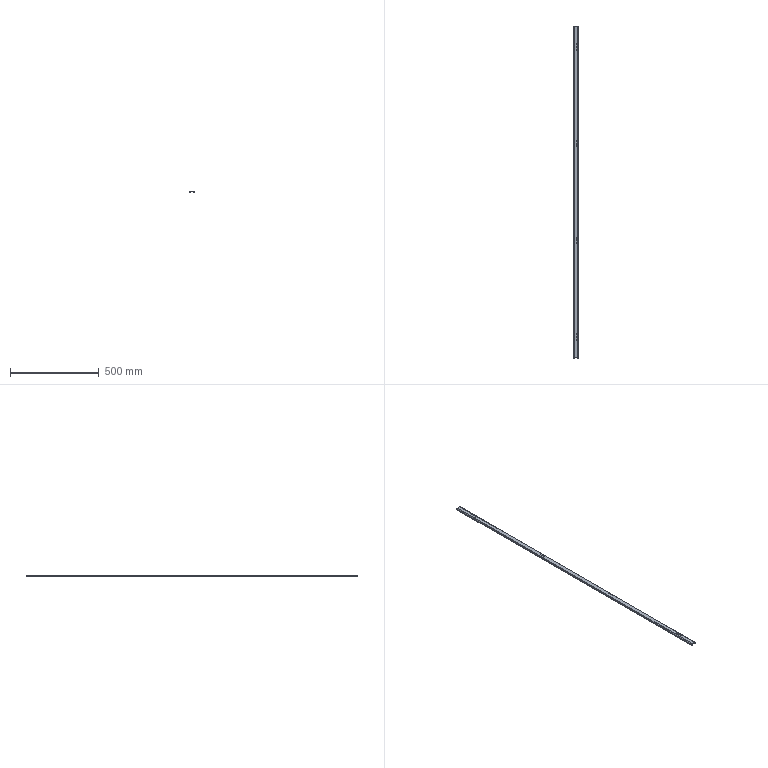Part | SolidWorks | features BaseBody 1 | 1 solid | 46 faces | box 27 x 1872 x 10 mm | volume 219826 mm3 | cylinder 28 | plane 18 | commonest cylinder face diameters 5.2 x24 1 x2 7 x2
STEP:
#1=CARTESIAN_POINT('',(1.9,-272.5,-3.));
#2=VERTEX_POINT('',#1);
#3=CARTESIAN_POINT('',(1.9,-272.5,0.));
#4=VERTEX_POINT('',#3);
#5=CARTESIAN_POINT('',(1.9,-272.5,-3.));
#6=DIRECTION('',(0.,0.,1.));
#7=VECTOR('',#6,1000.);
#8=LINE('',#5,#7);
#9=EDGE_CURVE('',#2,#4,#8,.T.);
#10=ORIENTED_EDGE('',*,*,#9,.F.);
#11=CARTESIAN_POINT('',(7.1,-272.5,-3.));
#12=VERTEX_POINT('',#11);
#13=CARTESIAN_POINT('',(4.5,-272.5,-3.));
#14=DIRECTION('',(0.,0.,1.));
#15=DIRECTION('',(1.,0.,0.));
#16=AXIS2_PLACEMENT_3D('',#13,#14,#15);
#17=CIRCLE('',#16,2.6);
#18=EDGE_CURVE('',#12,#2,#17,.T.);
#19=ORIENTED_EDGE('',*,*,#18,.F.);
#20=CARTESIAN_POINT('',(7.1,-272.5,0.));
#21=VERTEX_POINT('',#20);
#22=CARTESIAN_POINT('',(7.1,-272.5,-3.));
#23=DIRECTION('',(0.,0.,1.));
#24=VECTOR('',#23,1000.);
#25=LINE('',#22,#24);
#26=EDGE_CURVE('',#12,#21,#25,.T.);
#27=ORIENTED_EDGE('',*,*,#26,.T.);
#28=CARTESIAN_POINT('',(4.5,-272.5,0.));
#29=DIRECTION('',(0.,0.,1.));
#30=DIRECTION('',(1.,0.,0.));
#31=AXIS2_PLACEMENT_3D('',#28,#29,#30);
#32=CIRCLE('',#31,2.6);
#33=EDGE_CURVE('',#21,#4,#32,.T.);
#34=ORIENTED_EDGE('',*,*,#33,.T.);
#35=EDGE_LOOP('',(#10,#19,#27,#34));
#36=FACE_OUTER_BOUND('',#35,.T.);
#37=CARTESIAN_POINT('',(4.5,-272.5,-3.));
#38=DIRECTION('',(0.,0.,1.));
#39=DIRECTION('',(1.,0.,0.));
#40=AXIS2_PLACEMENT_3D('',#37,#38,#39);
#41=CYLINDRICAL_SURFACE('',#40,2.6);
#42=ADVANCED_FACE('',(#36),#41,.F.);
#43=CARTESIAN_POINT('',(1.9,-257.5,-3.));
#44=VERTEX_POINT('',#43);
#45=CARTESIAN_POINT('',(1.9,-257.5,0.));
#46=VERTEX_POINT('',#45);
#47=CARTESIAN_POINT('',(1.9,-257.5,-3.));
#48=DIRECTION('',(0.,0.,1.));
#49=VECTOR('',#48,1000.);
#50=LINE('',#47,#49);
#51=EDGE_CURVE('',#44,#46,#50,.T.);
#52=ORIENTED_EDGE('',*,*,#51,.F.);
#53=CARTESIAN_POINT('',(7.1,-257.5,-3.));
#54=VERTEX_POINT('',#53);
#55=CARTESIAN_POINT('',(4.5,-257.5,-3.));
#56=DIRECTION('',(0.,0.,1.));
#57=DIRECTION('',(1.,0.,0.));
#58=AXIS2_PLACEMENT_3D('',#55,#56,#57);
#59=CIRCLE('',#58,2.6);
#60=EDGE_CURVE('',#54,#44,#59,.T.);
#61=ORIENTED_EDGE('',*,*,#60,.F.);
#62=CARTESIAN_POINT('',(7.1,-257.5,0.));
#63=VERTEX_POINT('',#62);
#64=CARTESIAN_POINT('',(7.1,-257.5,-3.));
#65=DIRECTION('',(0.,0.,1.));
#66=VECTOR('',#65,1000.);
#67=LINE('',#64,#66);
#68=EDGE_CURVE('',#54,#63,#67,.T.);
#69=ORIENTED_EDGE('',*,*,#68,.T.);
#70=CARTESIAN_POINT('',(4.5,-257.5,0.));
#71=DIRECTION('',(0.,0.,1.));
#72=DIRECTION('',(1.,0.,0.));
#73=AXIS2_PLACEMENT_3D('',#70,#71,#72);
#74=CIRCLE('',#73,2.6);
#75=EDGE_CURVE('',#63,#46,#74,.T.);
#76=ORIENTED_EDGE('',*,*,#75,.T.);
#77=EDGE_LOOP('',(#52,#61,#69,#76));
#78=FACE_OUTER_BOUND('',#77,.T.);
#79=CARTESIAN_POINT('',(4.5,-257.5,-3.));
#80=DIRECTION('',(0.,0.,1.));
#81=DIRECTION('',(1.,0.,0.));
#82=AXIS2_PLACEMENT_3D('',#79,#80,#81);
#83=CYLINDRICAL_SURFACE('',#82,2.6);
#84=ADVANCED_FACE('',(#78),#83,.F.);
#85=CARTESIAN_POINT('',(1.9,-287.5,-3.));
#86=VERTEX_POINT('',#85);
#87=CARTESIAN_POINT('',(1.9,-287.5,0.));
#88=VERTEX_POINT('',#87);
#89=CARTESIAN_POINT('',(1.9,-287.5,-3.));
#90=DIRECTION('',(0.,0.,1.));
#91=VECTOR('',#90,1000.);
#92=LINE('',#89,#91);
#93=EDGE_CURVE('',#86,#88,#92,.T.);
#94=ORIENTED_EDGE('',*,*,#93,.F.);
#95=CARTESIAN_POINT('',(7.1,-287.5,-3.));
#96=VERTEX_POINT('',#95);
#97=CARTESIAN_POINT('',(4.5,-287.5,-3.));
#98=DIRECTION('',(0.,0.,1.));
#99=DIRECTION('',(1.,0.,0.));
#100=AXIS2_PLACEMENT_3D('',#97,#98,#99);
#101=CIRCLE('',#100,2.6);
#102=EDGE_CURVE('',#96,#86,#101,.T.);
#103=ORIENTED_EDGE('',*,*,#102,.F.);
#104=CARTESIAN_POINT('',(7.1,-287.5,0.));
#105=VERTEX_POINT('',#104);
#106=CARTESIAN_POINT('',(7.1,-287.5,-3.));
#107=DIRECTION('',(0.,0.,1.));
#108=VECTOR('',#107,1000.);
#109=LINE('',#106,#108);
#110=EDGE_CURVE('',#96,#105,#109,.T.);
#111=ORIENTED_EDGE('',*,*,#110,.T.);
#112=CARTESIAN_POINT('',(4.5,-287.5,0.));
#113=DIRECTION('',(0.,0.,1.));
#114=DIRECTION('',(1.,0.,0.));
#115=AXIS2_PLACEMENT_3D('',#112,#113,#114);
#116=CIRCLE('',#115,2.6);
#117=EDGE_CURVE('',#105,#88,#116,.T.);
#118=ORIENTED_EDGE('',*,*,#117,.T.);
#119=EDGE_LOOP('',(#94,#103,#111,#118));
#120=FACE_OUTER_BOUND('',#119,.T.);
#121=CARTESIAN_POINT('',(4.5,-287.5,-3.));
#122=DIRECTION('',(0.,0.,1.));
#123=DIRECTION('',(1.,0.,0.));
#124=AXIS2_PLACEMENT_3D('',#121,#122,#123);
#125=CYLINDRICAL_SURFACE('',#124,2.6);
#126=ADVANCED_FACE('',(#120),#125,.F.);
#127=CARTESIAN_POINT('',(1.9,-832.5,-3.));
#128=VERTEX_POINT('',#127);
#129=CARTESIAN_POINT('',(1.9,-832.5,0.));
#130=VERTEX_POINT('',#129);
#131=CARTESIAN_POINT('',(1.9,-832.5,-3.));
#132=DIRECTION('',(0.,0.,1.));
#133=VECTOR('',#132,1000.);
#134=LINE('',#131,#133);
#135=EDGE_CURVE('',#128,#130,#134,.T.);
#136=ORIENTED_EDGE('',*,*,#135,.F.);
#137=CARTESIAN_POINT('',(7.1,-832.5,-3.));
#138=VERTEX_POINT('',#137);
#139=CARTESIAN_POINT('',(4.5,-832.5,-3.));
#140=DIRECTION('',(0.,0.,1.));
#141=DIRECTION('',(1.,0.,0.));
#142=AXIS2_PLACEMENT_3D('',#139,#140,#141);
#143=CIRCLE('',#142,2.6);
#144=EDGE_CURVE('',#138,#128,#143,.T.);
#145=ORIENTED_EDGE('',*,*,#144,.F.);
#146=CARTESIAN_POINT('',(7.1,-832.5,0.));
#147=VERTEX_POINT('',#146);
#148=CARTESIAN_POINT('',(7.1,-832.5,-3.));
#149=DIRECTION('',(0.,0.,1.));
#150=VECTOR('',#149,1000.);
#151=LINE('',#148,#150);
#152=EDGE_CURVE('',#138,#147,#151,.T.);
#153=ORIENTED_EDGE('',*,*,#152,.T.);
#154=CARTESIAN_POINT('',(4.5,-832.5,0.));
#155=DIRECTION('',(0.,0.,1.));
#156=DIRECTION('',(1.,0.,0.));
#157=AXIS2_PLACEMENT_3D('',#154,#155,#156);
#158=CIRCLE('',#157,2.6);
#159=EDGE_CURVE('',#147,#130,#158,.T.);
#160=ORIENTED_EDGE('',*,*,#159,.T.);
#161=EDGE_LOOP('',(#136,#145,#153,#160));
#162=FACE_OUTER_BOUND('',#161,.T.);
#163=CARTESIAN_POINT('',(4.5,-832.5,-3.));
#164=DIRECTION('',(0.,0.,1.));
#165=DIRECTION('',(1.,0.,0.));
#166=AXIS2_PLACEMENT_3D('',#163,#164,#165);
#167=CYLINDRICAL_SURFACE('',#166,2.6);
#168=ADVANCED_FACE('',(#162),#167,.F.);
#169=CARTESIAN_POINT('',(1.9,-817.5,-3.));
#170=VERTEX_POINT('',#169);
#171=CARTESIAN_POINT('',(1.9,-817.5,0.));
#172=VERTEX_POINT('',#171);
#173=CARTESIAN_POINT('',(1.9,-817.5,-3.));
#174=DIRECTION('',(0.,0.,1.));
#175=VECTOR('',#174,1000.);
#176=LINE('',#173,#175);
#177=EDGE_CURVE('',#170,#172,#176,.T.);
#178=ORIENTED_EDGE('',*,*,#177,.F.);
#179=CARTESIAN_POINT('',(7.1,-817.5,-3.));
#180=VERTEX_POINT('',#179);
#181=CARTESIAN_POINT('',(4.5,-817.5,-3.));
#182=DIRECTION('',(0.,0.,1.));
#183=DIRECTION('',(1.,0.,0.));
#184=AXIS2_PLACEMENT_3D('',#181,#182,#183);
#185=CIRCLE('',#184,2.6);
#186=EDGE_CURVE('',#180,#170,#185,.T.);
#187=ORIENTED_EDGE('',*,*,#186,.F.);
#188=CARTESIAN_POINT('',(7.1,-817.5,0.));
#189=VERTEX_POINT('',#188);
#190=CARTESIAN_POINT('',(7.1,-817.5,-3.));
#191=DIRECTION('',(0.,0.,1.));
#192=VECTOR('',#191,1000.);
#193=LINE('',#190,#192);
#194=EDGE_CURVE('',#180,#189,#193,.T.);
#195=ORIENTED_EDGE('',*,*,#194,.T.);
#196=CARTESIAN_POINT('',(4.5,-817.5,0.));
#197=DIRECTION('',(0.,0.,1.));
#198=DIRECTION('',(1.,0.,0.));
#199=AXIS2_PLACEMENT_3D('',#196,#197,#198);
#200=CIRCLE('',#199,2.6);
#201=EDGE_CURVE('',#189,#172,#200,.T.);
#202=ORIENTED_EDGE('',*,*,#201,.T.);
#203=EDGE_LOOP('',(#178,#187,#195,#202));
#204=FACE_OUTER_BOUND('',#203,.T.);
#205=CARTESIAN_POINT('',(4.5,-817.5,-3.));
#206=DIRECTION('',(0.,0.,1.));
#207=DIRECTION('',(1.,0.,0.));
#208=AXIS2_PLACEMENT_3D('',#205,#206,#207);
#209=CYLINDRICAL_SURFACE('',#208,2.6);
#210=ADVANCED_FACE('',(#204),#209,.F.);
#211=CARTESIAN_POINT('',(1.9,-802.5,-3.));
#212=VERTEX_POINT('',#211);
#213=CARTESIAN_POINT('',(1.9,-802.5,0.));
#214=VERTEX_POINT('',#213);
#215=CARTESIAN_POINT('',(1.9,-802.5,-3.));
#216=DIRECTION('',(0.,0.,1.));
#217=VECTOR('',#216,1000.);
#218=LINE('',#215,#217);
#219=EDGE_CURVE('',#212,#214,#218,.T.);
#220=ORIENTED_EDGE('',*,*,#219,.F.);
#221=CARTESIAN_POINT('',(7.1,-802.5,-3.));
#222=VERTEX_POINT('',#221);
#223=CARTESIAN_POINT('',(4.5,-802.5,-3.));
#224=DIRECTION('',(0.,0.,1.));
#225=DIRECTION('',(1.,0.,0.));
#226=AXIS2_PLACEMENT_3D('',#223,#224,#225);
#227=CIRCLE('',#226,2.6);
#228=EDGE_CURVE('',#222,#212,#227,.T.);
#229=ORIENTED_EDGE('',*,*,#228,.F.);
#230=CARTESIAN_POINT('',(7.1,-802.5,0.));
#231=VERTEX_POINT('',#230);
#232=CARTESIAN_POINT('',(7.1,-802.5,-3.));
#233=DIRECTION('',(0.,0.,1.));
#234=VECTOR('',#233,1000.);
#235=LINE('',#232,#234);
#236=EDGE_CURVE('',#222,#231,#235,.T.);
#237=ORIENTED_EDGE('',*,*,#236,.T.);
#238=CARTESIAN_POINT('',(4.5,-802.5,0.));
#239=DIRECTION('',(0.,0.,1.));
#240=DIRECTION('',(1.,0.,0.));
#241=AXIS2_PLACEMENT_3D('',#238,#239,#240);
#242=CIRCLE('',#241,2.6);
#243=EDGE_CURVE('',#231,#214,#242,.T.);
#244=ORIENTED_EDGE('',*,*,#243,.T.);
#245=EDGE_LOOP('',(#220,#229,#237,#244));
#246=FACE_OUTER_BOUND('',#245,.T.);
#247=CARTESIAN_POINT('',(4.5,-802.5,-3.));
#248=DIRECTION('',(0.,0.,1.));
#249=DIRECTION('',(1.,0.,0.));
#250=AXIS2_PLACEMENT_3D('',#247,#248,#249);
#251=CYLINDRICAL_SURFACE('',#250,2.6);
#252=ADVANCED_FACE('',(#246),#251,.F.);
#253=CARTESIAN_POINT('',(-10.5,935.9,-10.));
#254=VERTEX_POINT('',#253);
#255=CARTESIAN_POINT('',(-10.5,-935.9,-10.));
#256=VERTEX_POINT('',#255);
#257=CARTESIAN_POINT('',(-10.5,-935.9,-10.));
#258=DIRECTION('',(0.,-1.,0.));
#259=VECTOR('',#258,1000.);
#260=LINE('',#257,#259);
#261=EDGE_CURVE('',#254,#256,#260,.T.);
#262=ORIENTED_EDGE('',*,*,#261,.T.);
#263=CARTESIAN_POINT('',(-13.5,-935.9,-10.));
#264=VERTEX_POINT('',#263);
#265=CARTESIAN_POINT('',(-13.5,-935.9,-10.));
#266=DIRECTION('',(1.,0.,0.));
#267=VECTOR('',#266,1000.);
#268=LINE('',#265,#267);
#269=EDGE_CURVE('',#264,#256,#268,.T.);
#270=ORIENTED_EDGE('',*,*,#269,.F.);
#271=CARTESIAN_POINT('',(-13.5,935.9,-10.));
#272=VERTEX_POINT('',#271);
#273=CARTESIAN_POINT('',(-13.5,0.,-10.));
#274=DIRECTION('',(0.,-1.,0.));
#275=VECTOR('',#274,1000.);
#276=LINE('',#273,#275);
#277=EDGE_CURVE('',#272,#264,#276,.T.);
#278=ORIENTED_EDGE('',*,*,#277,.F.);
#279=CARTESIAN_POINT('',(-13.5,935.9,-10.));
#280=DIRECTION('',(1.,0.,0.));
#281=VECTOR('',#280,1000.);
#282=LINE('',#279,#281);
#283=EDGE_CURVE('',#272,#254,#282,.T.);
#284=ORIENTED_EDGE('',*,*,#283,.T.);
#285=EDGE_LOOP('',(#262,#270,#278,#284));
#286=FACE_OUTER_BOUND('',#285,.T.);
#287=CARTESIAN_POINT('',(-13.5,-935.9,-10.));
#288=DIRECTION('',(0.,0.,1.));
#289=DIRECTION('',(1.,0.,0.));
#290=AXIS2_PLACEMENT_3D('',#287,#288,#289);
#291=PLANE('',#290);
#292=ADVANCED_FACE('',(#286),#291,.F.);
#293=CARTESIAN_POINT('',(-10.5,935.9,-3.5));
#294=VERTEX_POINT('',#293);
#295=CARTESIAN_POINT('',(-10.5,935.9,-10.));
#296=DIRECTION('',(0.,0.,-1.));
#297=VECTOR('',#296,1000.);
#298=LINE('',#295,#297);
#299=EDGE_CURVE('',#294,#254,#298,.T.);
#300=ORIENTED_EDGE('',*,*,#299,.F.);
#301=CARTESIAN_POINT('',(-10.5,-935.9,-3.5));
#302=VERTEX_POINT('',#301);
#303=CARTESIAN_POINT('',(-10.5,-935.9,-3.5));
#304=DIRECTION('',(0.,1.,0.));
#305=VECTOR('',#304,1000.);
#306=LINE('',#303,#305);
#307=EDGE_CURVE('',#302,#294,#306,.T.);
#308=ORIENTED_EDGE('',*,*,#307,.F.);
#309=CARTESIAN_POINT('',(-10.5,-935.9,-3.));
#310=DIRECTION('',(0.,0.,1.));
#311=VECTOR('',#310,1000.);
#312=LINE('',#309,#311);
#313=EDGE_CURVE('',#256,#302,#312,.T.);
#314=ORIENTED_EDGE('',*,*,#313,.F.);
#315=ORIENTED_EDGE('',*,*,#261,.F.);
#316=EDGE_LOOP('',(#300,#308,#314,#315));
#317=FACE_OUTER_BOUND('',#316,.T.);
#318=CARTESIAN_POINT('',(-10.5,0.,0.));
#319=DIRECTION('',(1.,0.,0.));
#320=DIRECTION('',(0.,0.,-1.));
#321=AXIS2_PLACEMENT_3D('',#318,#319,#320);
#322=PLANE('',#321);
#323=ADVANCED_FACE('',(#317),#322,.T.);
#324=CARTESIAN_POINT('',(-13.5,935.9,-3.5));
#325=VERTEX_POINT('',#324);
#326=CARTESIAN_POINT('',(-13.5,-935.9,-3.5));
#327=VERTEX_POINT('',#326);
#328=CARTESIAN_POINT('',(-13.5,-935.9,-3.5));
#329=DIRECTION('',(0.,-1.,0.));
#330=VECTOR('',#329,1000.);
#331=LINE('',#328,#330);
#332=EDGE_CURVE('',#325,#327,#331,.T.);
#333=ORIENTED_EDGE('',*,*,#332,.F.);
#334=CARTESIAN_POINT('',(-13.5,935.9,0.));
#335=DIRECTION('',(0.,0.,-1.));
#336=VECTOR('',#335,1000.);
#337=LINE('',#334,#336);
#338=EDGE_CURVE('',#325,#272,#337,.T.);
#339=ORIENTED_EDGE('',*,*,#338,.T.);
#340=ORIENTED_EDGE('',*,*,#277,.T.);
#341=CARTESIAN_POINT('',(-13.5,-935.9,0.));
#342=DIRECTION('',(0.,0.,1.));
#343=VECTOR('',#342,1000.);
#344=LINE('',#341,#343);
#345=EDGE_CURVE('',#264,#327,#344,.T.);
#346=ORIENTED_EDGE('',*,*,#345,.T.);
#347=EDGE_LOOP('',(#333,#339,#340,#346));
#348=FACE_OUTER_BOUND('',#347,.T.);
#349=CARTESIAN_POINT('',(-13.5,0.,0.));
#350=DIRECTION('',(1.,0.,0.));
#351=DIRECTION('',(0.,0.,-1.));
#352=AXIS2_PLACEMENT_3D('',#349,#350,#351);
#353=PLANE('',#352);
#354=ADVANCED_FACE('',(#348),#353,.F.);
#355=CARTESIAN_POINT('',(-13.5,-935.9,-3.5));
#356=DIRECTION('',(-1.,0.,0.));
#357=VECTOR('',#356,1000.);
#358=LINE('',#355,#357);
#359=EDGE_CURVE('',#302,#327,#358,.T.);
#360=ORIENTED_EDGE('',*,*,#359,.T.);
#361=ORIENTED_EDGE('',*,*,#345,.F.);
#362=ORIENTED_EDGE('',*,*,#269,.T.);
#363=ORIENTED_EDGE('',*,*,#313,.T.);
#364=EDGE_LOOP('',(#360,#361,#362,#363));
#365=FACE_OUTER_BOUND('',#364,.T.);
#366=CARTESIAN_POINT('',(-13.5,-935.9,-3.));
#367=DIRECTION('',(0.,1.,0.));
#368=DIRECTION('',(1.,0.,0.));
#369=AXIS2_PLACEMENT_3D('',#366,#367,#368);
#370=PLANE('',#369);
#371=ADVANCED_FACE('',(#365),#370,.F.);
#372=CARTESIAN_POINT('',(-10.5,935.9,-3.5));
#373=DIRECTION('',(-1.,0.,0.));
#374=VECTOR('',#373,1000.);
#375=LINE('',#372,#374);
#376=EDGE_CURVE('',#294,#325,#375,.T.);
#377=ORIENTED_EDGE('',*,*,#376,.F.);
#378=ORIENTED_EDGE('',*,*,#299,.T.);
#379=ORIENTED_EDGE('',*,*,#283,.F.);
#380=ORIENTED_EDGE('',*,*,#338,.F.);
#381=EDGE_LOOP('',(#377,#378,#379,#380));
#382=FACE_OUTER_BOUND('',#381,.T.);
#383=CARTESIAN_POINT('',(-13.5,935.9,-10.));
#384=DIRECTION('',(0.,-1.,0.));
#385=DIRECTION('',(0.,0.,-1.));
#386=AXIS2_PLACEMENT_3D('',#383,#384,#385);
#387=PLANE('',#386);
#388=ADVANCED_FACE('',(#382),#387,.F.);
#389=CARTESIAN_POINT('',(-10.,935.9,-3.));
#390=VERTEX_POINT('',#389);
#391=CARTESIAN_POINT('',(-10.,-935.9,-3.));
#392=VERTEX_POINT('',#391);
#393=CARTESIAN_POINT('',(-10.,935.9,-3.));
#394=DIRECTION('',(0.,-1.,0.));
#395=VECTOR('',#394,1000.);
#396=LINE('',#393,#395);
#397=EDGE_CURVE('',#390,#392,#396,.T.);
#398=ORIENTED_EDGE('',*,*,#397,.T.);
#399=CARTESIAN_POINT('',(-10.,-935.9,-3.5));
#400=DIRECTION('',(0.,-1.,0.));
#401=DIRECTION('',(0.,0.,1.));
#402=AXIS2_PLACEMENT_3D('',#399,#400,#401);
#403=CIRCLE('',#402,0.5);
#404=EDGE_CURVE('',#392,#302,#403,.T.);
#405=ORIENTED_EDGE('',*,*,#404,.T.);
#406=ORIENTED_EDGE('',*,*,#307,.T.);
#407=CARTESIAN_POINT('',(-10.,935.9,-3.5));
#408=DIRECTION('',(0.,1.,0.));
#409=DIRECTION('',(0.,0.,1.));
#410=AXIS2_PLACEMENT_3D('',#407,#408,#409);
#411=CIRCLE('',#410,0.5);
#412=EDGE_CURVE('',#294,#390,#411,.T.);
#413=ORIENTED_EDGE('',*,*,#412,.T.);
#414=EDGE_LOOP('',(#398,#405,#406,#413));
#415=FACE_OUTER_BOUND('',#414,.T.);
#416=CARTESIAN_POINT('',(-10.,935.9,-3.5));
#417=DIRECTION('',(0.,1.,0.));
#418=DIRECTION('',(-1.,0.,0.));
#419=AXIS2_PLACEMENT_3D('',#416,#417,#418);
#420=CYLINDRICAL_SURFACE('',#419,0.5);
#421=ADVANCED_FACE('',(#415),#420,.F.);
#422=CARTESIAN_POINT('',(-10.,935.9,0.));
#423=VERTEX_POINT('',#422);
#424=CARTESIAN_POINT('',(-10.,-935.9,0.));
#425=VERTEX_POINT('',#424);
#426=CARTESIAN_POINT('',(-10.,935.9,0.));
#427=DIRECTION('',(0.,-1.,0.));
#428=VECTOR('',#427,1000.);
#429=LINE('',#426,#428);
#430=EDGE_CURVE('',#423,#425,#429,.T.);
#431=ORIENTED_EDGE('',*,*,#430,.F.);
#432=CARTESIAN_POINT('',(-10.,935.9,-3.5));
#433=DIRECTION('',(0.,1.,0.));
#434=DIRECTION('',(0.,0.,1.));
#435=AXIS2_PLACEMENT_3D('',#432,#433,#434);
#436=CIRCLE('',#435,3.5);
#437=EDGE_CURVE('',#325,#423,#436,.T.);
#438=ORIENTED_EDGE('',*,*,#437,.F.);
#439=ORIENTED_EDGE('',*,*,#332,.T.);
#440=CARTESIAN_POINT('',(-10.,-935.9,-3.5));
#441=DIRECTION('',(0.,-1.,0.));
#442=DIRECTION('',(0.,0.,1.));
#443=AXIS2_PLACEMENT_3D('',#440,#441,#442);
#444=CIRCLE('',#443,3.5);
#445=EDGE_CURVE('',#425,#327,#444,.T.);
#446=ORIENTED_EDGE('',*,*,#445,.F.);
#447=EDGE_LOOP('',(#431,#438,#439,#446));
#448=FACE_OUTER_BOUND('',#447,.T.);
#449=CARTESIAN_POINT('',(-10.,935.9,-3.5));
#450=DIRECTION('',(0.,1.,0.));
#451=DIRECTION('',(-1.,0.,0.));
#452=AXIS2_PLACEMENT_3D('',#449,#450,#451);
#453=CYLINDRICAL_SURFACE('',#452,3.5);
#454=ADVANCED_FACE('',(#448),#453,.T.);
#455=ORIENTED_EDGE('',*,*,#412,.F.);
#456=ORIENTED_EDGE('',*,*,#376,.T.);
#457=ORIENTED_EDGE('',*,*,#437,.T.);
#458=CARTESIAN_POINT('',(-10.,935.9,-3.));
#459=DIRECTION('',(0.,0.,1.));
#460=VECTOR('',#459,1000.);
#461=LINE('',#458,#460);
#462=EDGE_CURVE('',#390,#423,#461,.T.);
#463=ORIENTED_EDGE('',*,*,#462,.F.);
#464=EDGE_LOOP('',(#455,#456,#457,#463));
#465=FACE_OUTER_BOUND('',#464,.T.);
#466=CARTESIAN_POINT('',(-10.,935.9,-3.5));
#467=DIRECTION('',(0.,-1.,0.));
#468=DIRECTION('',(0.,0.,-1.));
#469=AXIS2_PLACEMENT_3D('',#466,#467,#468);
#470=PLANE('',#469);
#471=ADVANCED_FACE('',(#465),#470,.F.);
#472=ORIENTED_EDGE('',*,*,#359,.F.);
#473=ORIENTED_EDGE('',*,*,#404,.F.);
#474=CARTESIAN_POINT('',(-10.,-935.9,-3.));
#475=DIRECTION('',(0.,0.,1.));
#476=VECTOR('',#475,1000.);
#477=LINE('',#474,#476);
#478=EDGE_CURVE('',#392,#425,#477,.T.);
#479=ORIENTED_EDGE('',*,*,#478,.T.);
#480=ORIENTED_EDGE('',*,*,#445,.T.);
#481=EDGE_LOOP('',(#472,#473,#479,#480));
#482=FACE_OUTER_BOUND('',#481,.T.);
#483=CARTESIAN_POINT('',(-10.,-935.9,-3.5));
#484=DIRECTION('',(0.,-1.,0.));
#485=DIRECTION('',(0.,0.,-1.));
#486=AXIS2_PLACEMENT_3D('',#483,#484,#485);
#487=PLANE('',#486);
#488=ADVANCED_FACE('',(#482),#487,.T.);
#489=CARTESIAN_POINT('',(10.5,-935.9,-10.));
#490=VERTEX_POINT('',#489);
#491=CARTESIAN_POINT('',(10.5,935.9,-10.));
#492=VERTEX_POINT('',#491);
#493=CARTESIAN_POINT('',(10.5,935.9,-10.));
#494=DIRECTION('',(0.,1.,0.));
#495=VECTOR('',#494,1000.);
#496=LINE('',#493,#495);
#497=EDGE_CURVE('',#490,#492,#496,.T.);
#498=ORIENTED_EDGE('',*,*,#497,.T.);
#499=CARTESIAN_POINT('',(13.5,935.9,-10.));
#500=VERTEX_POINT('',#499);
#501=CARTESIAN_POINT('',(13.5,935.9,-10.));
#502=DIRECTION('',(-1.,0.,0.));
#503=VECTOR('',#502,1000.);
#504=LINE('',#501,#503);
#505=EDGE_CURVE('',#500,#492,#504,.T.);
#506=ORIENTED_EDGE('',*,*,#505,.F.);
#507=CARTESIAN_POINT('',(13.5,-935.9,-10.));
#508=VERTEX_POINT('',#507);
#509=CARTESIAN_POINT('',(13.5,0.,-10.));
#510=DIRECTION('',(0.,1.,0.));
#511=VECTOR('',#510,1000.);
#512=LINE('',#509,#511);
#513=EDGE_CURVE('',#508,#500,#512,.T.);
#514=ORIENTED_EDGE('',*,*,#513,.F.);
#515=CARTESIAN_POINT('',(13.5,-935.9,-10.));
#516=DIRECTION('',(-1.,0.,0.));
#517=VECTOR('',#516,1000.);
#518=LINE('',#515,#517);
#519=EDGE_CURVE('',#508,#490,#518,.T.);
#520=ORIENTED_EDGE('',*,*,#519,.T.);
#521=EDGE_LOOP('',(#498,#506,#514,#520));
#522=FACE_OUTER_BOUND('',#521,.T.);
#523=CARTESIAN_POINT('',(13.5,935.9,-10.));
#524=DIRECTION('',(0.,0.,1.));
#525=DIRECTION('',(1.,0.,0.));
#526=AXIS2_PLACEMENT_3D('',#523,#524,#525);
#527=PLANE('',#526);
#528=ADVANCED_FACE('',(#522),#527,.F.);
#529=CARTESIAN_POINT('',(10.5,-935.9,-3.5));
#530=VERTEX_POINT('',#529);
#531=CARTESIAN_POINT('',(10.5,-935.9,-10.));
#532=DIRECTION('',(0.,0.,-1.));
#533=VECTOR('',#532,1000.);
#534=LINE('',#531,#533);
#535=EDGE_CURVE('',#530,#490,#534,.T.);
#536=ORIENTED_EDGE('',*,*,#535,.F.);
#537=CARTESIAN_POINT('',(10.5,935.9,-3.5));
#538=VERTEX_POINT('',#537);
#539=CARTESIAN_POINT('',(10.5,935.9,-3.5));
#540=DIRECTION('',(0.,-1.,0.));
#541=VECTOR('',#540,1000.);
#542=LINE('',#539,#541);
#543=EDGE_CURVE('',#538,#530,#542,.T.);
#544=ORIENTED_EDGE('',*,*,#543,.F.);
#545=CARTESIAN_POINT('',(10.5,935.9,-3.));
#546=DIRECTION('',(0.,0.,1.));
#547=VECTOR('',#546,1000.);
#548=LINE('',#545,#547);
#549=EDGE_CURVE('',#492,#538,#548,.T.);
#550=ORIENTED_EDGE('',*,*,#549,.F.);
#551=ORIENTED_EDGE('',*,*,#497,.F.);
#552=EDGE_LOOP('',(#536,#544,#550,#551));
#553=FACE_OUTER_BOUND('',#552,.T.);
#554=CARTESIAN_POINT('',(10.5,0.,0.));
#555=DIRECTION('',(-1.,0.,0.));
#556=DIRECTION('',(0.,0.,1.));
#557=AXIS2_PLACEMENT_3D('',#554,#555,#556);
#558=PLANE('',#557);
#559=ADVANCED_FACE('',(#553),#558,.T.);
#560=CARTESIAN_POINT('',(13.5,-935.9,-3.5));
#561=VERTEX_POINT('',#560);
#562=CARTESIAN_POINT('',(13.5,935.9,-3.5));
#563=VERTEX_POINT('',#562);
#564=CARTESIAN_POINT('',(13.5,935.9,-3.5));
#565=DIRECTION('',(0.,1.,0.));
#566=VECTOR('',#565,1000.);
#567=LINE('',#564,#566);
#568=EDGE_CURVE('',#561,#563,#567,.T.);
#569=ORIENTED_EDGE('',*,*,#568,.F.);
#570=CARTESIAN_POINT('',(13.5,-935.9,0.));
#571=DIRECTION('',(0.,0.,-1.));
#572=VECTOR('',#571,1000.);
#573=LINE('',#570,#572);
#574=EDGE_CURVE('',#561,#508,#573,.T.);
#575=ORIENTED_EDGE('',*,*,#574,.T.);
#576=ORIENTED_EDGE('',*,*,#513,.T.);
#577=CARTESIAN_POINT('',(13.5,935.9,0.));
#578=DIRECTION('',(0.,0.,1.));
#579=VECTOR('',#578,1000.);
#580=LINE('',#577,#579);
#581=EDGE_CURVE('',#500,#563,#580,.T.);
#582=ORIENTED_EDGE('',*,*,#581,.T.);
#583=EDGE_LOOP('',(#569,#575,#576,#582));
#584=FACE_OUTER_BOUND('',#583,.T.);
#585=CARTESIAN_POINT('',(13.5,0.,0.));
#586=DIRECTION('',(-1.,0.,0.));
#587=DIRECTION('',(0.,0.,1.));
#588=AXIS2_PLACEMENT_3D('',#585,#586,#587);
#589=PLANE('',#588);
#590=ADVANCED_FACE('',(#584),#589,.F.);
#591=CARTESIAN_POINT('',(13.5,935.9,-3.5));
#592=DIRECTION('',(1.,0.,0.));
#593=VECTOR('',#592,1000.);
#594=LINE('',#591,#593);
#595=EDGE_CURVE('',#538,#563,#594,.T.);
#596=ORIENTED_EDGE('',*,*,#595,.T.);
#597=ORIENTED_EDGE('',*,*,#581,.F.);
#598=ORIENTED_EDGE('',*,*,#505,.T.);
#599=ORIENTED_EDGE('',*,*,#549,.T.);
#600=EDGE_LOOP('',(#596,#597,#598,#599));
#601=FACE_OUTER_BOUND('',#600,.T.);
#602=CARTESIAN_POINT('',(13.5,935.9,-3.));
#603=DIRECTION('',(0.,-1.,0.));
#604=DIRECTION('',(0.,0.,-1.));
#605=AXIS2_PLACEMENT_3D('',#602,#603,#604);
#606=PLANE('',#605);
#607=ADVANCED_FACE('',(#601),#606,.F.);
#608=CARTESIAN_POINT('',(10.5,-935.9,-3.5));
#609=DIRECTION('',(1.,0.,0.));
#610=VECTOR('',#609,1000.);
#611=LINE('',#608,#610);
#612=EDGE_CURVE('',#530,#561,#611,.T.);
#613=ORIENTED_EDGE('',*,*,#612,.F.);
#614=ORIENTED_EDGE('',*,*,#535,.T.);
#615=ORIENTED_EDGE('',*,*,#519,.F.);
#616=ORIENTED_EDGE('',*,*,#574,.F.);
#617=EDGE_LOOP('',(#613,#614,#615,#616));
#618=FACE_OUTER_BOUND('',#617,.T.);
#619=CARTESIAN_POINT('',(13.5,-935.9,-10.));
#620=DIRECTION('',(0.,1.,0.));
#621=DIRECTION('',(1.,0.,0.));
#622=AXIS2_PLACEMENT_3D('',#619,#620,#621);
#623=PLANE('',#622);
#624=ADVANCED_FACE('',(#618),#623,.F.);
#625=CARTESIAN_POINT('',(10.,-935.9,-3.));
#626=VERTEX_POINT('',#625);
#627=CARTESIAN_POINT('',(10.,935.9,-3.));
#628=VERTEX_POINT('',#627);
#629=CARTESIAN_POINT('',(10.,-935.9,-3.));
#630=DIRECTION('',(0.,1.,0.));
#631=VECTOR('',#630,1000.);
#632=LINE('',#629,#631);
#633=EDGE_CURVE('',#626,#628,#632,.T.);
#634=ORIENTED_EDGE('',*,*,#633,.T.);
#635=CARTESIAN_POINT('',(10.,935.9,-3.5));
#636=DIRECTION('',(0.,1.,0.));
#637=DIRECTION('',(0.,0.,-1.));
#638=AXIS2_PLACEMENT_3D('',#635,#636,#637);
#639=CIRCLE('',#638,0.5);
#640=EDGE_CURVE('',#628,#538,#639,.T.);
#641=ORIENTED_EDGE('',*,*,#640,.T.);
#642=ORIENTED_EDGE('',*,*,#543,.T.);
#643=CARTESIAN_POINT('',(10.,-935.9,-3.5));
#644=DIRECTION('',(0.,-1.,0.));
#645=DIRECTION('',(0.,0.,-1.));
#646=AXIS2_PLACEMENT_3D('',#643,#644,#645);
#647=CIRCLE('',#646,0.5);
#648=EDGE_CURVE('',#530,#626,#647,.T.);
#649=ORIENTED_EDGE('',*,*,#648,.T.);
#650=EDGE_LOOP('',(#634,#641,#642,#649));
#651=FACE_OUTER_BOUND('',#650,.T.);
#652=CARTESIAN_POINT('',(10.,-935.9,-3.5));
#653=DIRECTION('',(0.,-1.,0.));
#654=DIRECTION('',(1.,0.,0.));
#655=AXIS2_PLACEMENT_3D('',#652,#653,#654);
#656=CYLINDRICAL_SURFACE('',#655,0.5);
#657=ADVANCED_FACE('',(#651),#656,.F.);
#658=CARTESIAN_POINT('',(10.,-935.9,0.));
#659=VERTEX_POINT('',#658);
#660=CARTESIAN_POINT('',(10.,935.9,0.));
#661=VERTEX_POINT('',#660);
#662=CARTESIAN_POINT('',(10.,-935.9,0.));
#663=DIRECTION('',(0.,1.,0.));
#664=VECTOR('',#663,1000.);
#665=LINE('',#662,#664);
#666=EDGE_CURVE('',#659,#661,#665,.T.);
#667=ORIENTED_EDGE('',*,*,#666,.F.);
#668=CARTESIAN_POINT('',(10.,-935.9,-3.5));
#669=DIRECTION('',(0.,-1.,0.));
#670=DIRECTION('',(0.,0.,-1.));
#671=AXIS2_PLACEMENT_3D('',#668,#669,#670);
#672=CIRCLE('',#671,3.5);
#673=EDGE_CURVE('',#561,#659,#672,.T.);
#674=ORIENTED_EDGE('',*,*,#673,.F.);
#675=ORIENTED_EDGE('',*,*,#568,.T.);
#676=CARTESIAN_POINT('',(10.,935.9,-3.5));
#677=DIRECTION('',(0.,1.,0.));
#678=DIRECTION('',(0.,0.,-1.));
#679=AXIS2_PLACEMENT_3D('',#676,#677,#678);
#680=CIRCLE('',#679,3.5);
#681=EDGE_CURVE('',#661,#563,#680,.T.);
#682=ORIENTED_EDGE('',*,*,#681,.F.);
#683=EDGE_LOOP('',(#667,#674,#675,#682));
#684=FACE_OUTER_BOUND('',#683,.T.);
#685=CARTESIAN_POINT('',(10.,-935.9,-3.5));
#686=DIRECTION('',(0.,-1.,0.));
#687=DIRECTION('',(1.,0.,0.));
#688=AXIS2_PLACEMENT_3D('',#685,#686,#687);
#689=CYLINDRICAL_SURFACE('',#688,3.5);
#690=ADVANCED_FACE('',(#684),#689,.T.);
#691=ORIENTED_EDGE('',*,*,#648,.F.);
#692=ORIENTED_EDGE('',*,*,#612,.T.);
#693=ORIENTED_EDGE('',*,*,#673,.T.);
#694=CARTESIAN_POINT('',(10.,-935.9,-3.));
#695=DIRECTION('',(0.,0.,1.));
#696=VECTOR('',#695,1000.);
#697=LINE('',#694,#696);
#698=EDGE_CURVE('',#626,#659,#697,.T.);
#699=ORIENTED_EDGE('',*,*,#698,.F.);
#700=EDGE_LOOP('',(#691,#692,#693,#699));
#701=FACE_OUTER_BOUND('',#700,.T.);
#702=CARTESIAN_POINT('',(10.,-935.9,-3.5));
#703=DIRECTION('',(0.,1.,0.));
#704=DIRECTION('',(1.,0.,0.));
#705=AXIS2_PLACEMENT_3D('',#702,#703,#704);
#706=PLANE('',#705);
#707=ADVANCED_FACE('',(#701),#706,.F.);
#708=ORIENTED_EDGE('',*,*,#595,.F.);
#709=ORIENTED_EDGE('',*,*,#640,.F.);
#710=CARTESIAN_POINT('',(10.,935.9,-3.));
#711=DIRECTION('',(0.,0.,1.));
#712=VECTOR('',#711,1000.);
#713=LINE('',#710,#712);
#714=EDGE_CURVE('',#628,#661,#713,.T.);
#715=ORIENTED_EDGE('',*,*,#714,.T.);
#716=ORIENTED_EDGE('',*,*,#681,.T.);
#717=EDGE_LOOP('',(#708,#709,#715,#716));
#718=FACE_OUTER_BOUND('',#717,.T.);
#719=CARTESIAN_POINT('',(10.,935.9,-3.5));
#720=DIRECTION('',(0.,1.,0.));
#721=DIRECTION('',(1.,0.,0.));
#722=AXIS2_PLACEMENT_3D('',#719,#720,#721);
#723=PLANE('',#722);
#724=ADVANCED_FACE('',(#718),#723,.T.);
#725=ORIENTED_EDGE('',*,*,#478,.F.);
#726=CARTESIAN_POINT('',(13.5,-935.9,-3.));
#727=DIRECTION('',(1.,0.,0.));
#728=VECTOR('',#727,1000.);
#729=LINE('',#726,#728);
#730=EDGE_CURVE('',#392,#626,#729,.T.);
#731=ORIENTED_EDGE('',*,*,#730,.T.);
#732=ORIENTED_EDGE('',*,*,#698,.T.);
#733=CARTESIAN_POINT('',(13.5,-935.9,0.));
#734=DIRECTION('',(1.,0.,0.));
#735=VECTOR('',#734,1000.);
#736=LINE('',#733,#735);
#737=EDGE_CURVE('',#425,#659,#736,.T.);
#738=ORIENTED_EDGE('',*,*,#737,.F.);
#739=EDGE_LOOP('',(#725,#731,#732,#738));
#740=FACE_OUTER_BOUND('',#739,.T.);
#741=CARTESIAN_POINT('',(13.5,-935.9,-3.));
#742=DIRECTION('',(0.,-1.,0.));
#743=DIRECTION('',(0.,0.,-1.));
#744=AXIS2_PLACEMENT_3D('',#741,#742,#743);
#745=PLANE('',#744);
#746=ADVANCED_FACE('',(#740),#745,.T.);
#747=CARTESIAN_POINT('',(13.5,935.9,-3.));
#748=DIRECTION('',(-1.,0.,0.));
#749=VECTOR('',#748,1000.);
#750=LINE('',#747,#749);
#751=EDGE_CURVE('',#628,#390,#750,.T.);
#752=ORIENTED_EDGE('',*,*,#751,.T.);
#753=ORIENTED_EDGE('',*,*,#462,.T.);
#754=CARTESIAN_POINT('',(13.5,935.9,0.));
#755=DIRECTION('',(-1.,0.,0.));
#756=VECTOR('',#755,1000.);
#757=LINE('',#754,#756);
#758=EDGE_CURVE('',#661,#423,#757,.T.);
#759=ORIENTED_EDGE('',*,*,#758,.F.);
#760=ORIENTED_EDGE('',*,*,#714,.F.);
#761=EDGE_LOOP('',(#752,#753,#759,#760));
#762=FACE_OUTER_BOUND('',#761,.T.);
#763=CARTESIAN_POINT('',(13.5,935.9,-3.));
#764=DIRECTION('',(0.,1.,0.));
#765=DIRECTION('',(1.,0.,0.));
#766=AXIS2_PLACEMENT_3D('',#763,#764,#765);
#767=PLANE('',#766);
#768=ADVANCED_FACE('',(#762),#767,.T.);
#769=CARTESIAN_POINT('',(7.1,817.5,0.));
#770=VERTEX_POINT('',#769);
#771=CARTESIAN_POINT('',(1.9,817.5,0.));
#772=VERTEX_POINT('',#771);
#773=CARTESIAN_POINT('',(4.5,817.5,0.));
#774=DIRECTION('',(0.,0.,1.));
#775=DIRECTION('',(1.,0.,0.));
#776=AXIS2_PLACEMENT_3D('',#773,#774,#775);
#777=CIRCLE('',#776,2.6);
#778=EDGE_CURVE('',#770,#772,#777,.T.);
#779=ORIENTED_EDGE('',*,*,#778,.F.);
#780=CARTESIAN_POINT('',(4.5,817.5,0.));
#781=DIRECTION('',(0.,0.,1.));
#782=DIRECTION('',(1.,0.,0.));
#783=AXIS2_PLACEMENT_3D('',#780,#781,#782);
#784=CIRCLE('',#783,2.6);
#785=EDGE_CURVE('',#772,#770,#784,.T.);
#786=ORIENTED_EDGE('',*,*,#785,.F.);
#787=EDGE_LOOP('',(#779,#786));
#788=FACE_BOUND('',#787,.T.);
#789=CARTESIAN_POINT('',(7.1,272.5,0.));
#790=VERTEX_POINT('',#789);
#791=CARTESIAN_POINT('',(1.9,272.5,0.));
#792=VERTEX_POINT('',#791);
#793=CARTESIAN_POINT('',(4.5,272.5,0.));
#794=DIRECTION('',(0.,0.,1.));
#795=DIRECTION('',(1.,0.,0.));
#796=AXIS2_PLACEMENT_3D('',#793,#794,#795);
#797=CIRCLE('',#796,2.6);
#798=EDGE_CURVE('',#790,#792,#797,.T.);
#799=ORIENTED_EDGE('',*,*,#798,.F.);
#800=CARTESIAN_POINT('',(4.5,272.5,0.));
#801=DIRECTION('',(0.,0.,1.));
#802=DIRECTION('',(1.,0.,0.));
#803=AXIS2_PLACEMENT_3D('',#800,#801,#802);
#804=CIRCLE('',#803,2.6);
#805=EDGE_CURVE('',#792,#790,#804,.T.);
#806=ORIENTED_EDGE('',*,*,#805,.F.);
#807=EDGE_LOOP('',(#799,#806));
#808=FACE_BOUND('',#807,.T.);
#809=CARTESIAN_POINT('',(7.1,832.5,0.));
#810=VERTEX_POINT('',#809);
#811=CARTESIAN_POINT('',(1.9,832.5,0.));
#812=VERTEX_POINT('',#811);
#813=CARTESIAN_POINT('',(4.5,832.5,0.));
#814=DIRECTION('',(0.,0.,1.));
#815=DIRECTION('',(1.,0.,0.));
#816=AXIS2_PLACEMENT_3D('',#813,#814,#815);
#817=CIRCLE('',#816,2.6);
#818=EDGE_CURVE('',#810,#812,#817,.T.);
#819=ORIENTED_EDGE('',*,*,#818,.F.);
#820=CARTESIAN_POINT('',(4.5,832.5,0.));
#821=DIRECTION('',(0.,0.,1.));
#822=DIRECTION('',(1.,0.,0.));
#823=AXIS2_PLACEMENT_3D('',#820,#821,#822);
#824=CIRCLE('',#823,2.6);
#825=EDGE_CURVE('',#812,#810,#824,.T.);
#826=ORIENTED_EDGE('',*,*,#825,.F.);
#827=EDGE_LOOP('',(#819,#826));
#828=FACE_BOUND('',#827,.T.);
#829=CARTESIAN_POINT('',(7.1,287.5,0.));
#830=VERTEX_POINT('',#829);
#831=CARTESIAN_POINT('',(1.9,287.5,0.));
#832=VERTEX_POINT('',#831);
#833=CARTESIAN_POINT('',(4.5,287.5,0.));
#834=DIRECTION('',(0.,0.,1.));
#835=DIRECTION('',(1.,0.,0.));
#836=AXIS2_PLACEMENT_3D('',#833,#834,#835);
#837=CIRCLE('',#836,2.6);
#838=EDGE_CURVE('',#830,#832,#837,.T.);
#839=ORIENTED_EDGE('',*,*,#838,.F.);
#840=CARTESIAN_POINT('',(4.5,287.5,0.));
#841=DIRECTION('',(0.,0.,1.));
#842=DIRECTION('',(1.,0.,0.));
#843=AXIS2_PLACEMENT_3D('',#840,#841,#842);
#844=CIRCLE('',#843,2.6);
#845=EDGE_CURVE('',#832,#830,#844,.T.);
#846=ORIENTED_EDGE('',*,*,#845,.F.);
#847=EDGE_LOOP('',(#839,#846));
#848=FACE_BOUND('',#847,.T.);
#849=CARTESIAN_POINT('',(7.1,802.5,0.));
#850=VERTEX_POINT('',#849);
#851=CARTESIAN_POINT('',(1.9,802.5,0.));
#852=VERTEX_POINT('',#851);
#853=CARTESIAN_POINT('',(4.5,802.5,0.));
#854=DIRECTION('',(0.,0.,1.));
#855=DIRECTION('',(1.,0.,0.));
#856=AXIS2_PLACEMENT_3D('',#853,#854,#855);
#857=CIRCLE('',#856,2.6);
#858=EDGE_CURVE('',#850,#852,#857,.T.);
#859=ORIENTED_EDGE('',*,*,#858,.F.);
#860=CARTESIAN_POINT('',(4.5,802.5,0.));
#861=DIRECTION('',(0.,0.,1.));
#862=DIRECTION('',(1.,0.,0.));
#863=AXIS2_PLACEMENT_3D('',#860,#861,#862);
#864=CIRCLE('',#863,2.6);
#865=EDGE_CURVE('',#852,#850,#864,.T.);
#866=ORIENTED_EDGE('',*,*,#865,.F.);
#867=EDGE_LOOP('',(#859,#866));
#868=FACE_BOUND('',#867,.T.);
#869=CARTESIAN_POINT('',(7.1,257.5,0.));
#870=VERTEX_POINT('',#869);
#871=CARTESIAN_POINT('',(1.9,257.5,0.));
#872=VERTEX_POINT('',#871);
#873=CARTESIAN_POINT('',(4.5,257.5,0.));
#874=DIRECTION('',(0.,0.,1.));
#875=DIRECTION('',(1.,0.,0.));
#876=AXIS2_PLACEMENT_3D('',#873,#874,#875);
#877=CIRCLE('',#876,2.6);
#878=EDGE_CURVE('',#870,#872,#877,.T.);
#879=ORIENTED_EDGE('',*,*,#878,.F.);
#880=CARTESIAN_POINT('',(4.5,257.5,0.));
#881=DIRECTION('',(0.,0.,1.));
#882=DIRECTION('',(1.,0.,0.));
#883=AXIS2_PLACEMENT_3D('',#880,#881,#882);
#884=CIRCLE('',#883,2.6);
#885=EDGE_CURVE('',#872,#870,#884,.T.);
#886=ORIENTED_EDGE('',*,*,#885,.F.);
#887=EDGE_LOOP('',(#879,#886));
#888=FACE_BOUND('',#887,.T.);
#889=ORIENTED_EDGE('',*,*,#243,.F.);
#890=CARTESIAN_POINT('',(4.5,-802.5,0.));
#891=DIRECTION('',(0.,0.,1.));
#892=DIRECTION('',(1.,0.,0.));
#893=AXIS2_PLACEMENT_3D('',#890,#891,#892);
#894=CIRCLE('',#893,2.6);
#895=EDGE_CURVE('',#214,#231,#894,.T.);
#896=ORIENTED_EDGE('',*,*,#895,.F.);
#897=EDGE_LOOP('',(#889,#896));
#898=FACE_BOUND('',#897,.T.);
#899=ORIENTED_EDGE('',*,*,#201,.F.);
#900=CARTESIAN_POINT('',(4.5,-817.5,0.));
#901=DIRECTION('',(0.,0.,1.));
#902=DIRECTION('',(1.,0.,0.));
#903=AXIS2_PLACEMENT_3D('',#900,#901,#902);
#904=CIRCLE('',#903,2.6);
#905=EDGE_CURVE('',#172,#189,#904,.T.);
#906=ORIENTED_EDGE('',*,*,#905,.F.);
#907=EDGE_LOOP('',(#899,#906));
#908=FACE_BOUND('',#907,.T.);
#909=ORIENTED_EDGE('',*,*,#159,.F.);
#910=CARTESIAN_POINT('',(4.5,-832.5,0.));
#911=DIRECTION('',(0.,0.,1.));
#912=DIRECTION('',(1.,0.,0.));
#913=AXIS2_PLACEMENT_3D('',#910,#911,#912);
#914=CIRCLE('',#913,2.6);
#915=EDGE_CURVE('',#130,#147,#914,.T.);
#916=ORIENTED_EDGE('',*,*,#915,.F.);
#917=EDGE_LOOP('',(#909,#916));
#918=FACE_BOUND('',#917,.T.);
#919=ORIENTED_EDGE('',*,*,#117,.F.);
#920=CARTESIAN_POINT('',(4.5,-287.5,0.));
#921=DIRECTION('',(0.,0.,1.));
#922=DIRECTION('',(1.,0.,0.));
#923=AXIS2_PLACEMENT_3D('',#920,#921,#922);
#924=CIRCLE('',#923,2.6);
#925=EDGE_CURVE('',#88,#105,#924,.T.);
#926=ORIENTED_EDGE('',*,*,#925,.F.);
#927=EDGE_LOOP('',(#919,#926));
#928=FACE_BOUND('',#927,.T.);
#929=ORIENTED_EDGE('',*,*,#75,.F.);
#930=CARTESIAN_POINT('',(4.5,-257.5,0.));
#931=DIRECTION('',(0.,0.,1.));
#932=DIRECTION('',(1.,0.,0.));
#933=AXIS2_PLACEMENT_3D('',#930,#931,#932);
#934=CIRCLE('',#933,2.6);
#935=EDGE_CURVE('',#46,#63,#934,.T.);
#936=ORIENTED_EDGE('',*,*,#935,.F.);
#937=EDGE_LOOP('',(#929,#936));
#938=FACE_BOUND('',#937,.T.);
#939=ORIENTED_EDGE('',*,*,#33,.F.);
#940=CARTESIAN_POINT('',(4.5,-272.5,0.));
#941=DIRECTION('',(0.,0.,1.));
#942=DIRECTION('',(1.,0.,0.));
#943=AXIS2_PLACEMENT_3D('',#940,#941,#942);
#944=CIRCLE('',#943,2.6);
#945=EDGE_CURVE('',#4,#21,#944,.T.);
#946=ORIENTED_EDGE('',*,*,#945,.F.);
#947=EDGE_LOOP('',(#939,#946));
#948=FACE_BOUND('',#947,.T.);
#949=ORIENTED_EDGE('',*,*,#430,.T.);
#950=ORIENTED_EDGE('',*,*,#737,.T.);
#951=ORIENTED_EDGE('',*,*,#666,.T.);
#952=ORIENTED_EDGE('',*,*,#758,.T.);
#953=EDGE_LOOP('',(#949,#950,#951,#952));
#954=FACE_OUTER_BOUND('',#953,.T.);
#955=CARTESIAN_POINT('',(0.,0.,0.));
#956=DIRECTION('',(0.,0.,-1.));
#957=DIRECTION('',(0.,-1.,0.));
#958=AXIS2_PLACEMENT_3D('',#955,#956,#957);
#959=PLANE('',#958);
#960=ADVANCED_FACE('',(#788,#808,#828,#848,#868,#888,#898,#908,#918,#928,#938,#948,#954),#959,.F.);
#961=CARTESIAN_POINT('',(7.1,817.5,-3.));
#962=VERTEX_POINT('',#961);
#963=CARTESIAN_POINT('',(1.9,817.5,-3.));
#964=VERTEX_POINT('',#963);
#965=CARTESIAN_POINT('',(4.5,817.5,-3.));
#966=DIRECTION('',(0.,0.,1.));
#967=DIRECTION('',(1.,0.,0.));
#968=AXIS2_PLACEMENT_3D('',#965,#966,#967);
#969=CIRCLE('',#968,2.6);
#970=EDGE_CURVE('',#962,#964,#969,.T.);
#971=ORIENTED_EDGE('',*,*,#970,.T.);
#972=CARTESIAN_POINT('',(4.5,817.5,-3.));
#973=DIRECTION('',(0.,0.,1.));
#974=DIRECTION('',(1.,0.,0.));
#975=AXIS2_PLACEMENT_3D('',#972,#973,#974);
#976=CIRCLE('',#975,2.6);
#977=EDGE_CURVE('',#964,#962,#976,.T.);
#978=ORIENTED_EDGE('',*,*,#977,.T.);
#979=EDGE_LOOP('',(#971,#978));
#980=FACE_BOUND('',#979,.T.);
#981=CARTESIAN_POINT('',(7.1,272.5,-3.));
#982=VERTEX_POINT('',#981);
#983=CARTESIAN_POINT('',(1.9,272.5,-3.));
#984=VERTEX_POINT('',#983);
#985=CARTESIAN_POINT('',(4.5,272.5,-3.));
#986=DIRECTION('',(0.,0.,1.));
#987=DIRECTION('',(1.,0.,0.));
#988=AXIS2_PLACEMENT_3D('',#985,#986,#987);
#989=CIRCLE('',#988,2.6);
#990=EDGE_CURVE('',#982,#984,#989,.T.);
#991=ORIENTED_EDGE('',*,*,#990,.T.);
#992=CARTESIAN_POINT('',(4.5,272.5,-3.));
#993=DIRECTION('',(0.,0.,1.));
#994=DIRECTION('',(1.,0.,0.));
#995=AXIS2_PLACEMENT_3D('',#992,#993,#994);
#996=CIRCLE('',#995,2.6);
#997=EDGE_CURVE('',#984,#982,#996,.T.);
#998=ORIENTED_EDGE('',*,*,#997,.T.);
#999=EDGE_LOOP('',(#991,#998));
#1000=FACE_BOUND('',#999,.T.);
#1001=CARTESIAN_POINT('',(7.1,832.5,-3.));
#1002=VERTEX_POINT('',#1001);
#1003=CARTESIAN_POINT('',(1.9,832.5,-3.));
#1004=VERTEX_POINT('',#1003);
#1005=CARTESIAN_POINT('',(4.5,832.5,-3.));
#1006=DIRECTION('',(0.,0.,1.));
#1007=DIRECTION('',(1.,0.,0.));
#1008=AXIS2_PLACEMENT_3D('',#1005,#1006,#1007);
#1009=CIRCLE('',#1008,2.6);
#1010=EDGE_CURVE('',#1002,#1004,#1009,.T.);
#1011=ORIENTED_EDGE('',*,*,#1010,.T.);
#1012=CARTESIAN_POINT('',(4.5,832.5,-3.));
#1013=DIRECTION('',(0.,0.,1.));
#1014=DIRECTION('',(1.,0.,0.));
#1015=AXIS2_PLACEMENT_3D('',#1012,#1013,#1014);
#1016=CIRCLE('',#1015,2.6);
#1017=EDGE_CURVE('',#1004,#1002,#1016,.T.);
#1018=ORIENTED_EDGE('',*,*,#1017,.T.);
#1019=EDGE_LOOP('',(#1011,#1018));
#1020=FACE_BOUND('',#1019,.T.);
#1021=CARTESIAN_POINT('',(7.1,287.5,-3.));
#1022=VERTEX_POINT('',#1021);
#1023=CARTESIAN_POINT('',(1.9,287.5,-3.));
#1024=VERTEX_POINT('',#1023);
#1025=CARTESIAN_POINT('',(4.5,287.5,-3.));
#1026=DIRECTION('',(0.,0.,1.));
#1027=DIRECTION('',(1.,0.,0.));
#1028=AXIS2_PLACEMENT_3D('',#1025,#1026,#1027);
#1029=CIRCLE('',#1028,2.6);
#1030=EDGE_CURVE('',#1022,#1024,#1029,.T.);
#1031=ORIENTED_EDGE('',*,*,#1030,.T.);
#1032=CARTESIAN_POINT('',(4.5,287.5,-3.));
#1033=DIRECTION('',(0.,0.,1.));
#1034=DIRECTION('',(1.,0.,0.));
#1035=AXIS2_PLACEMENT_3D('',#1032,#1033,#1034);
#1036=CIRCLE('',#1035,2.6);
#1037=EDGE_CURVE('',#1024,#1022,#1036,.T.);
#1038=ORIENTED_EDGE('',*,*,#1037,.T.);
#1039=EDGE_LOOP('',(#1031,#1038));
#1040=FACE_BOUND('',#1039,.T.);
#1041=CARTESIAN_POINT('',(7.1,802.5,-3.));
#1042=VERTEX_POINT('',#1041);
#1043=CARTESIAN_POINT('',(1.9,802.5,-3.));
#1044=VERTEX_POINT('',#1043);
#1045=CARTESIAN_POINT('',(4.5,802.5,-3.));
#1046=DIRECTION('',(0.,0.,1.));
#1047=DIRECTION('',(1.,0.,0.));
#1048=AXIS2_PLACEMENT_3D('',#1045,#1046,#1047);
#1049=CIRCLE('',#1048,2.6);
#1050=EDGE_CURVE('',#1042,#1044,#1049,.T.);
#1051=ORIENTED_EDGE('',*,*,#1050,.T.);
#1052=CARTESIAN_POINT('',(4.5,802.5,-3.));
#1053=DIRECTION('',(0.,0.,1.));
#1054=DIRECTION('',(1.,0.,0.));
#1055=AXIS2_PLACEMENT_3D('',#1052,#1053,#1054);
#1056=CIRCLE('',#1055,2.6);
#1057=EDGE_CURVE('',#1044,#1042,#1056,.T.);
#1058=ORIENTED_EDGE('',*,*,#1057,.T.);
#1059=EDGE_LOOP('',(#1051,#1058));
#1060=FACE_BOUND('',#1059,.T.);
#1061=CARTESIAN_POINT('',(7.1,257.5,-3.));
#1062=VERTEX_POINT('',#1061);
#1063=CARTESIAN_POINT('',(1.9,257.5,-3.));
#1064=VERTEX_POINT('',#1063);
#1065=CARTESIAN_POINT('',(4.5,257.5,-3.));
#1066=DIRECTION('',(0.,0.,1.));
#1067=DIRECTION('',(1.,0.,0.));
#1068=AXIS2_PLACEMENT_3D('',#1065,#1066,#1067);
#1069=CIRCLE('',#1068,2.6);
#1070=EDGE_CURVE('',#1062,#1064,#1069,.T.);
#1071=ORIENTED_EDGE('',*,*,#1070,.T.);
#1072=CARTESIAN_POINT('',(4.5,257.5,-3.));
#1073=DIRECTION('',(0.,0.,1.));
#1074=DIRECTION('',(1.,0.,0.));
#1075=AXIS2_PLACEMENT_3D('',#1072,#1073,#1074);
#1076=CIRCLE('',#1075,2.6);
#1077=EDGE_CURVE('',#1064,#1062,#1076,.T.);
#1078=ORIENTED_EDGE('',*,*,#1077,.T.);
#1079=EDGE_LOOP('',(#1071,#1078));
#1080=FACE_BOUND('',#1079,.T.);
#1081=ORIENTED_EDGE('',*,*,#228,.T.);
#1082=CARTESIAN_POINT('',(4.5,-802.5,-3.));
#1083=DIRECTION('',(0.,0.,1.));
#1084=DIRECTION('',(1.,0.,0.));
#1085=AXIS2_PLACEMENT_3D('',#1082,#1083,#1084);
#1086=CIRCLE('',#1085,2.6);
#1087=EDGE_CURVE('',#212,#222,#1086,.T.);
#1088=ORIENTED_EDGE('',*,*,#1087,.T.);
#1089=EDGE_LOOP('',(#1081,#1088));
#1090=FACE_BOUND('',#1089,.T.);
#1091=ORIENTED_EDGE('',*,*,#186,.T.);
#1092=CARTESIAN_POINT('',(4.5,-817.5,-3.));
#1093=DIRECTION('',(0.,0.,1.));
#1094=DIRECTION('',(1.,0.,0.));
#1095=AXIS2_PLACEMENT_3D('',#1092,#1093,#1094);
#1096=CIRCLE('',#1095,2.6);
#1097=EDGE_CURVE('',#170,#180,#1096,.T.);
#1098=ORIENTED_EDGE('',*,*,#1097,.T.);
#1099=EDGE_LOOP('',(#1091,#1098));
#1100=FACE_BOUND('',#1099,.T.);
#1101=ORIENTED_EDGE('',*,*,#144,.T.);
#1102=CARTESIAN_POINT('',(4.5,-832.5,-3.));
#1103=DIRECTION('',(0.,0.,1.));
#1104=DIRECTION('',(1.,0.,0.));
#1105=AXIS2_PLACEMENT_3D('',#1102,#1103,#1104);
#1106=CIRCLE('',#1105,2.6);
#1107=EDGE_CURVE('',#128,#138,#1106,.T.);
#1108=ORIENTED_EDGE('',*,*,#1107,.T.);
#1109=EDGE_LOOP('',(#1101,#1108));
#1110=FACE_BOUND('',#1109,.T.);
#1111=ORIENTED_EDGE('',*,*,#102,.T.);
#1112=CARTESIAN_POINT('',(4.5,-287.5,-3.));
#1113=DIRECTION('',(0.,0.,1.));
#1114=DIRECTION('',(1.,0.,0.));
#1115=AXIS2_PLACEMENT_3D('',#1112,#1113,#1114);
#1116=CIRCLE('',#1115,2.6);
#1117=EDGE_CURVE('',#86,#96,#1116,.T.);
#1118=ORIENTED_EDGE('',*,*,#1117,.T.);
#1119=EDGE_LOOP('',(#1111,#1118));
#1120=FACE_BOUND('',#1119,.T.);
#1121=ORIENTED_EDGE('',*,*,#60,.T.);
#1122=CARTESIAN_POINT('',(4.5,-257.5,-3.));
#1123=DIRECTION('',(0.,0.,1.));
#1124=DIRECTION('',(1.,0.,0.));
#1125=AXIS2_PLACEMENT_3D('',#1122,#1123,#1124);
#1126=CIRCLE('',#1125,2.6);
#1127=EDGE_CURVE('',#44,#54,#1126,.T.);
#1128=ORIENTED_EDGE('',*,*,#1127,.T.);
#1129=EDGE_LOOP('',(#1121,#1128));
#1130=FACE_BOUND('',#1129,.T.);
#1131=ORIENTED_EDGE('',*,*,#18,.T.);
#1132=CARTESIAN_POINT('',(4.5,-272.5,-3.));
#1133=DIRECTION('',(0.,0.,1.));
#1134=DIRECTION('',(1.,0.,0.));
#1135=AXIS2_PLACEMENT_3D('',#1132,#1133,#1134);
#1136=CIRCLE('',#1135,2.6);
#1137=EDGE_CURVE('',#2,#12,#1136,.T.);
#1138=ORIENTED_EDGE('',*,*,#1137,.T.);
#1139=EDGE_LOOP('',(#1131,#1138));
#1140=FACE_BOUND('',#1139,.T.);
#1141=ORIENTED_EDGE('',*,*,#730,.F.);
#1142=ORIENTED_EDGE('',*,*,#397,.F.);
#1143=ORIENTED_EDGE('',*,*,#751,.F.);
#1144=ORIENTED_EDGE('',*,*,#633,.F.);
#1145=EDGE_LOOP('',(#1141,#1142,#1143,#1144));
#1146=FACE_OUTER_BOUND('',#1145,.T.);
#1147=CARTESIAN_POINT('',(0.,0.,-3.));
#1148=DIRECTION('',(0.,0.,-1.));
#1149=DIRECTION('',(0.,-1.,0.));
#1150=AXIS2_PLACEMENT_3D('',#1147,#1148,#1149);
#1151=PLANE('',#1150);
#1152=ADVANCED_FACE('',(#980,#1000,#1020,#1040,#1060,#1080,#1090,#1100,#1110,#1120,#1130,#1140,#1146),#1151,.T.);
#1153=CARTESIAN_POINT('',(1.9,257.5,-3.));
#1154=DIRECTION('',(0.,0.,1.));
#1155=VECTOR('',#1154,1000.);
#1156=LINE('',#1153,#1155);
#1157=EDGE_CURVE('',#1064,#872,#1156,.T.);
#1158=ORIENTED_EDGE('',*,*,#1157,.F.);
#1159=ORIENTED_EDGE('',*,*,#1070,.F.);
#1160=CARTESIAN_POINT('',(7.1,257.5,-3.));
#1161=DIRECTION('',(0.,0.,1.));
#1162=VECTOR('',#1161,1000.);
#1163=LINE('',#1160,#1162);
#1164=EDGE_CURVE('',#1062,#870,#1163,.T.);
#1165=ORIENTED_EDGE('',*,*,#1164,.T.);
#1166=ORIENTED_EDGE('',*,*,#878,.T.);
#1167=EDGE_LOOP('',(#1158,#1159,#1165,#1166));
#1168=FACE_OUTER_BOUND('',#1167,.T.);
#1169=CARTESIAN_POINT('',(4.5,257.5,-3.));
#1170=DIRECTION('',(0.,0.,1.));
#1171=DIRECTION('',(1.,0.,0.));
#1172=AXIS2_PLACEMENT_3D('',#1169,#1170,#1171);
#1173=CYLINDRICAL_SURFACE('',#1172,2.6);
#1174=ADVANCED_FACE('',(#1168),#1173,.F.);
#1175=CARTESIAN_POINT('',(1.9,802.5,-3.));
#1176=DIRECTION('',(0.,0.,1.));
#1177=VECTOR('',#1176,1000.);
#1178=LINE('',#1175,#1177);
#1179=EDGE_CURVE('',#1044,#852,#1178,.T.);
#1180=ORIENTED_EDGE('',*,*,#1179,.F.);
#1181=ORIENTED_EDGE('',*,*,#1050,.F.);
#1182=CARTESIAN_POINT('',(7.1,802.5,-3.));
#1183=DIRECTION('',(0.,0.,1.));
#1184=VECTOR('',#1183,1000.);
#1185=LINE('',#1182,#1184);
#1186=EDGE_CURVE('',#1042,#850,#1185,.T.);
#1187=ORIENTED_EDGE('',*,*,#1186,.T.);
#1188=ORIENTED_EDGE('',*,*,#858,.T.);
#1189=EDGE_LOOP('',(#1180,#1181,#1187,#1188));
#1190=FACE_OUTER_BOUND('',#1189,.T.);
#1191=CARTESIAN_POINT('',(4.5,802.5,-3.));
#1192=DIRECTION('',(0.,0.,1.));
#1193=DIRECTION('',(1.,0.,0.));
#1194=AXIS2_PLACEMENT_3D('',#1191,#1192,#1193);
#1195=CYLINDRICAL_SURFACE('',#1194,2.6);
#1196=ADVANCED_FACE('',(#1190),#1195,.F.);
#1197=CARTESIAN_POINT('',(1.9,287.5,-3.));
#1198=DIRECTION('',(0.,0.,1.));
#1199=VECTOR('',#1198,1000.);
#1200=LINE('',#1197,#1199);
#1201=EDGE_CURVE('',#1024,#832,#1200,.T.);
#1202=ORIENTED_EDGE('',*,*,#1201,.F.);
#1203=ORIENTED_EDGE('',*,*,#1030,.F.);
#1204=CARTESIAN_POINT('',(7.1,287.5,-3.));
#1205=DIRECTION('',(0.,0.,1.));
#1206=VECTOR('',#1205,1000.);
#1207=LINE('',#1204,#1206);
#1208=EDGE_CURVE('',#1022,#830,#1207,.T.);
#1209=ORIENTED_EDGE('',*,*,#1208,.T.);
#1210=ORIENTED_EDGE('',*,*,#838,.T.);
#1211=EDGE_LOOP('',(#1202,#1203,#1209,#1210));
#1212=FACE_OUTER_BOUND('',#1211,.T.);
#1213=CARTESIAN_POINT('',(4.5,287.5,-3.));
#1214=DIRECTION('',(0.,0.,1.));
#1215=DIRECTION('',(1.,0.,0.));
#1216=AXIS2_PLACEMENT_3D('',#1213,#1214,#1215);
#1217=CYLINDRICAL_SURFACE('',#1216,2.6);
#1218=ADVANCED_FACE('',(#1212),#1217,.F.);
#1219=CARTESIAN_POINT('',(1.9,832.5,-3.));
#1220=DIRECTION('',(0.,0.,1.));
#1221=VECTOR('',#1220,1000.);
#1222=LINE('',#1219,#1221);
#1223=EDGE_CURVE('',#1004,#812,#1222,.T.);
#1224=ORIENTED_EDGE('',*,*,#1223,.F.);
#1225=ORIENTED_EDGE('',*,*,#1010,.F.);
#1226=CARTESIAN_POINT('',(7.1,832.5,-3.));
#1227=DIRECTION('',(0.,0.,1.));
#1228=VECTOR('',#1227,1000.);
#1229=LINE('',#1226,#1228);
#1230=EDGE_CURVE('',#1002,#810,#1229,.T.);
#1231=ORIENTED_EDGE('',*,*,#1230,.T.);
#1232=ORIENTED_EDGE('',*,*,#818,.T.);
#1233=EDGE_LOOP('',(#1224,#1225,#1231,#1232));
#1234=FACE_OUTER_BOUND('',#1233,.T.);
#1235=CARTESIAN_POINT('',(4.5,832.5,-3.));
#1236=DIRECTION('',(0.,0.,1.));
#1237=DIRECTION('',(1.,0.,0.));
#1238=AXIS2_PLACEMENT_3D('',#1235,#1236,#1237);
#1239=CYLINDRICAL_SURFACE('',#1238,2.6);
#1240=ADVANCED_FACE('',(#1234),#1239,.F.);
#1241=CARTESIAN_POINT('',(1.9,272.5,-3.));
#1242=DIRECTION('',(0.,0.,1.));
#1243=VECTOR('',#1242,1000.);
#1244=LINE('',#1241,#1243);
#1245=EDGE_CURVE('',#984,#792,#1244,.T.);
#1246=ORIENTED_EDGE('',*,*,#1245,.F.);
#1247=ORIENTED_EDGE('',*,*,#990,.F.);
#1248=CARTESIAN_POINT('',(7.1,272.5,-3.));
#1249=DIRECTION('',(0.,0.,1.));
#1250=VECTOR('',#1249,1000.);
#1251=LINE('',#1248,#1250);
#1252=EDGE_CURVE('',#982,#790,#1251,.T.);
#1253=ORIENTED_EDGE('',*,*,#1252,.T.);
#1254=ORIENTED_EDGE('',*,*,#798,.T.);
#1255=EDGE_LOOP('',(#1246,#1247,#1253,#1254));
#1256=FACE_OUTER_BOUND('',#1255,.T.);
#1257=CARTESIAN_POINT('',(4.5,272.5,-3.));
#1258=DIRECTION('',(0.,0.,1.));
#1259=DIRECTION('',(1.,0.,0.));
#1260=AXIS2_PLACEMENT_3D('',#1257,#1258,#1259);
#1261=CYLINDRICAL_SURFACE('',#1260,2.6);
#1262=ADVANCED_FACE('',(#1256),#1261,.F.);
#1263=CARTESIAN_POINT('',(1.9,817.5,-3.));
#1264=DIRECTION('',(0.,0.,1.));
#1265=VECTOR('',#1264,1000.);
#1266=LINE('',#1263,#1265);
#1267=EDGE_CURVE('',#964,#772,#1266,.T.);
#1268=ORIENTED_EDGE('',*,*,#1267,.F.);
#1269=ORIENTED_EDGE('',*,*,#970,.F.);
#1270=CARTESIAN_POINT('',(7.1,817.5,-3.));
#1271=DIRECTION('',(0.,0.,1.));
#1272=VECTOR('',#1271,1000.);
#1273=LINE('',#1270,#1272);
#1274=EDGE_CURVE('',#962,#770,#1273,.T.);
#1275=ORIENTED_EDGE('',*,*,#1274,.T.);
#1276=ORIENTED_EDGE('',*,*,#778,.T.);
#1277=EDGE_LOOP('',(#1268,#1269,#1275,#1276));
#1278=FACE_OUTER_BOUND('',#1277,.T.);
#1279=CARTESIAN_POINT('',(4.5,817.5,-3.));
#1280=DIRECTION('',(0.,0.,1.));
#1281=DIRECTION('',(1.,0.,0.));
#1282=AXIS2_PLACEMENT_3D('',#1279,#1280,#1281);
#1283=CYLINDRICAL_SURFACE('',#1282,2.6);
#1284=ADVANCED_FACE('',(#1278),#1283,.F.);
#1285=ORIENTED_EDGE('',*,*,#977,.F.);
#1286=ORIENTED_EDGE('',*,*,#1267,.T.);
#1287=ORIENTED_EDGE('',*,*,#785,.T.);
#1288=ORIENTED_EDGE('',*,*,#1274,.F.);
#1289=EDGE_LOOP('',(#1285,#1286,#1287,#1288));
#1290=FACE_OUTER_BOUND('',#1289,.T.);
#1291=CARTESIAN_POINT('',(4.5,817.5,-3.));
#1292=DIRECTION('',(0.,0.,1.));
#1293=DIRECTION('',(1.,0.,0.));
#1294=AXIS2_PLACEMENT_3D('',#1291,#1292,#1293);
#1295=CYLINDRICAL_SURFACE('',#1294,2.6);
#1296=ADVANCED_FACE('',(#1290),#1295,.F.);
#1297=ORIENTED_EDGE('',*,*,#997,.F.);
#1298=ORIENTED_EDGE('',*,*,#1245,.T.);
#1299=ORIENTED_EDGE('',*,*,#805,.T.);
#1300=ORIENTED_EDGE('',*,*,#1252,.F.);
#1301=EDGE_LOOP('',(#1297,#1298,#1299,#1300));
#1302=FACE_OUTER_BOUND('',#1301,.T.);
#1303=CARTESIAN_POINT('',(4.5,272.5,-3.));
#1304=DIRECTION('',(0.,0.,1.));
#1305=DIRECTION('',(1.,0.,0.));
#1306=AXIS2_PLACEMENT_3D('',#1303,#1304,#1305);
#1307=CYLINDRICAL_SURFACE('',#1306,2.6);
#1308=ADVANCED_FACE('',(#1302),#1307,.F.);
#1309=ORIENTED_EDGE('',*,*,#1017,.F.);
#1310=ORIENTED_EDGE('',*,*,#1223,.T.);
#1311=ORIENTED_EDGE('',*,*,#825,.T.);
#1312=ORIENTED_EDGE('',*,*,#1230,.F.);
#1313=EDGE_LOOP('',(#1309,#1310,#1311,#1312));
#1314=FACE_OUTER_BOUND('',#1313,.T.);
#1315=CARTESIAN_POINT('',(4.5,832.5,-3.));
#1316=DIRECTION('',(0.,0.,1.));
#1317=DIRECTION('',(1.,0.,0.));
#1318=AXIS2_PLACEMENT_3D('',#1315,#1316,#1317);
#1319=CYLINDRICAL_SURFACE('',#1318,2.6);
#1320=ADVANCED_FACE('',(#1314),#1319,.F.);
#1321=ORIENTED_EDGE('',*,*,#1037,.F.);
#1322=ORIENTED_EDGE('',*,*,#1201,.T.);
#1323=ORIENTED_EDGE('',*,*,#845,.T.);
#1324=ORIENTED_EDGE('',*,*,#1208,.F.);
#1325=EDGE_LOOP('',(#1321,#1322,#1323,#1324));
#1326=FACE_OUTER_BOUND('',#1325,.T.);
#1327=CARTESIAN_POINT('',(4.5,287.5,-3.));
#1328=DIRECTION('',(0.,0.,1.));
#1329=DIRECTION('',(1.,0.,0.));
#1330=AXIS2_PLACEMENT_3D('',#1327,#1328,#1329);
#1331=CYLINDRICAL_SURFACE('',#1330,2.6);
#1332=ADVANCED_FACE('',(#1326),#1331,.F.);
#1333=ORIENTED_EDGE('',*,*,#1057,.F.);
#1334=ORIENTED_EDGE('',*,*,#1179,.T.);
#1335=ORIENTED_EDGE('',*,*,#865,.T.);
#1336=ORIENTED_EDGE('',*,*,#1186,.F.);
#1337=EDGE_LOOP('',(#1333,#1334,#1335,#1336));
#1338=FACE_OUTER_BOUND('',#1337,.T.);
#1339=CARTESIAN_POINT('',(4.5,802.5,-3.));
#1340=DIRECTION('',(0.,0.,1.));
#1341=DIRECTION('',(1.,0.,0.));
#1342=AXIS2_PLACEMENT_3D('',#1339,#1340,#1341);
#1343=CYLINDRICAL_SURFACE('',#1342,2.6);
#1344=ADVANCED_FACE('',(#1338),#1343,.F.);
#1345=ORIENTED_EDGE('',*,*,#1077,.F.);
#1346=ORIENTED_EDGE('',*,*,#1157,.T.);
#1347=ORIENTED_EDGE('',*,*,#885,.T.);
#1348=ORIENTED_EDGE('',*,*,#1164,.F.);
#1349=EDGE_LOOP('',(#1345,#1346,#1347,#1348));
#1350=FACE_OUTER_BOUND('',#1349,.T.);
#1351=CARTESIAN_POINT('',(4.5,257.5,-3.));
#1352=DIRECTION('',(0.,0.,1.));
#1353=DIRECTION('',(1.,0.,0.));
#1354=AXIS2_PLACEMENT_3D('',#1351,#1352,#1353);
#1355=CYLINDRICAL_SURFACE('',#1354,2.6);
#1356=ADVANCED_FACE('',(#1350),#1355,.F.);
#1357=ORIENTED_EDGE('',*,*,#1087,.F.);
#1358=ORIENTED_EDGE('',*,*,#219,.T.);
#1359=ORIENTED_EDGE('',*,*,#895,.T.);
#1360=ORIENTED_EDGE('',*,*,#236,.F.);
#1361=EDGE_LOOP('',(#1357,#1358,#1359,#1360));
#1362=FACE_OUTER_BOUND('',#1361,.T.);
#1363=CARTESIAN_POINT('',(4.5,-802.5,-3.));
#1364=DIRECTION('',(0.,0.,1.));
#1365=DIRECTION('',(1.,0.,0.));
#1366=AXIS2_PLACEMENT_3D('',#1363,#1364,#1365);
#1367=CYLINDRICAL_SURFACE('',#1366,2.6);
#1368=ADVANCED_FACE('',(#1362),#1367,.F.);
#1369=ORIENTED_EDGE('',*,*,#1097,.F.);
#1370=ORIENTED_EDGE('',*,*,#177,.T.);
#1371=ORIENTED_EDGE('',*,*,#905,.T.);
#1372=ORIENTED_EDGE('',*,*,#194,.F.);
#1373=EDGE_LOOP('',(#1369,#1370,#1371,#1372));
#1374=FACE_OUTER_BOUND('',#1373,.T.);
#1375=CARTESIAN_POINT('',(4.5,-817.5,-3.));
#1376=DIRECTION('',(0.,0.,1.));
#1377=DIRECTION('',(1.,0.,0.));
#1378=AXIS2_PLACEMENT_3D('',#1375,#1376,#1377);
#1379=CYLINDRICAL_SURFACE('',#1378,2.6);
#1380=ADVANCED_FACE('',(#1374),#1379,.F.);
#1381=ORIENTED_EDGE('',*,*,#1107,.F.);
#1382=ORIENTED_EDGE('',*,*,#135,.T.);
#1383=ORIENTED_EDGE('',*,*,#915,.T.);
#1384=ORIENTED_EDGE('',*,*,#152,.F.);
#1385=EDGE_LOOP('',(#1381,#1382,#1383,#1384));
#1386=FACE_OUTER_BOUND('',#1385,.T.);
#1387=CARTESIAN_POINT('',(4.5,-832.5,-3.));
#1388=DIRECTION('',(0.,0.,1.));
#1389=DIRECTION('',(1.,0.,0.));
#1390=AXIS2_PLACEMENT_3D('',#1387,#1388,#1389);
#1391=CYLINDRICAL_SURFACE('',#1390,2.6);
#1392=ADVANCED_FACE('',(#1386),#1391,.F.);
#1393=ORIENTED_EDGE('',*,*,#1117,.F.);
#1394=ORIENTED_EDGE('',*,*,#93,.T.);
#1395=ORIENTED_EDGE('',*,*,#925,.T.);
#1396=ORIENTED_EDGE('',*,*,#110,.F.);
#1397=EDGE_LOOP('',(#1393,#1394,#1395,#1396));
#1398=FACE_OUTER_BOUND('',#1397,.T.);
#1399=CARTESIAN_POINT('',(4.5,-287.5,-3.));
#1400=DIRECTION('',(0.,0.,1.));
#1401=DIRECTION('',(1.,0.,0.));
#1402=AXIS2_PLACEMENT_3D('',#1399,#1400,#1401);
#1403=CYLINDRICAL_SURFACE('',#1402,2.6);
#1404=ADVANCED_FACE('',(#1398),#1403,.F.);
#1405=ORIENTED_EDGE('',*,*,#1127,.F.);
#1406=ORIENTED_EDGE('',*,*,#51,.T.);
#1407=ORIENTED_EDGE('',*,*,#935,.T.);
#1408=ORIENTED_EDGE('',*,*,#68,.F.);
#1409=EDGE_LOOP('',(#1405,#1406,#1407,#1408));
#1410=FACE_OUTER_BOUND('',#1409,.T.);
#1411=CARTESIAN_POINT('',(4.5,-257.5,-3.));
#1412=DIRECTION('',(0.,0.,1.));
#1413=DIRECTION('',(1.,0.,0.));
#1414=AXIS2_PLACEMENT_3D('',#1411,#1412,#1413);
#1415=CYLINDRICAL_SURFACE('',#1414,2.6);
#1416=ADVANCED_FACE('',(#1410),#1415,.F.);
#1417=ORIENTED_EDGE('',*,*,#1137,.F.);
#1418=ORIENTED_EDGE('',*,*,#9,.T.);
#1419=ORIENTED_EDGE('',*,*,#945,.T.);
#1420=ORIENTED_EDGE('',*,*,#26,.F.);
#1421=EDGE_LOOP('',(#1417,#1418,#1419,#1420));
#1422=FACE_OUTER_BOUND('',#1421,.T.);
#1423=CARTESIAN_POINT('',(4.5,-272.5,-3.));
#1424=DIRECTION('',(0.,0.,1.));
#1425=DIRECTION('',(1.,0.,0.));
#1426=AXIS2_PLACEMENT_3D('',#1423,#1424,#1425);
#1427=CYLINDRICAL_SURFACE('',#1426,2.6);
#1428=ADVANCED_FACE('',(#1422),#1427,.F.);
#1429=CLOSED_SHELL('',(#42,#84,#126,#168,#210,#252,#292,#323,#354,#371,#388,#421,#454,#471,#488,#528,#559,#590,#607,#624,#657,#690,#707,#724,#746,#768,#960,#1152,#1174,#1196,#1218,#1240,#1262,#1284,#1296,#1308,#1320,#1332,#1344,#1356,#1368,#1380,#1392,#1404,#1416,#1428));
#1430=MANIFOLD_SOLID_BREP('',#1429);
#1431=CARTESIAN_POINT('',(0.,0.,0.));
#1432=DIRECTION('',(0.,0.,1.));
#1433=DIRECTION('',(1.,0.,0.));
#1434=AXIS2_PLACEMENT_3D('',#1431,#1432,#1433);
#1435=(LENGTH_UNIT()NAMED_UNIT(*)SI_UNIT(.MILLI.,.METRE.));
#1436=UNCERTAINTY_MEASURE_WITH_UNIT(LENGTH_MEASURE(0.00001),#1435,'','');
#1437=(NAMED_UNIT(*)PLANE_ANGLE_UNIT()SI_UNIT($,.RADIAN.));
#1438=(NAMED_UNIT(*)SI_UNIT($,.STERADIAN.)SOLID_ANGLE_UNIT());
#1439=(GEOMETRIC_REPRESENTATION_CONTEXT(3)GLOBAL_UNCERTAINTY_ASSIGNED_CONTEXT((#1436))GLOBAL_UNIT_ASSIGNED_CONTEXT((#1435,#1437,#1438))REPRESENTATION_CONTEXT('',''));
#1440=ADVANCED_BREP_SHAPE_REPRESENTATION('',(#1430,#1434),#1439);